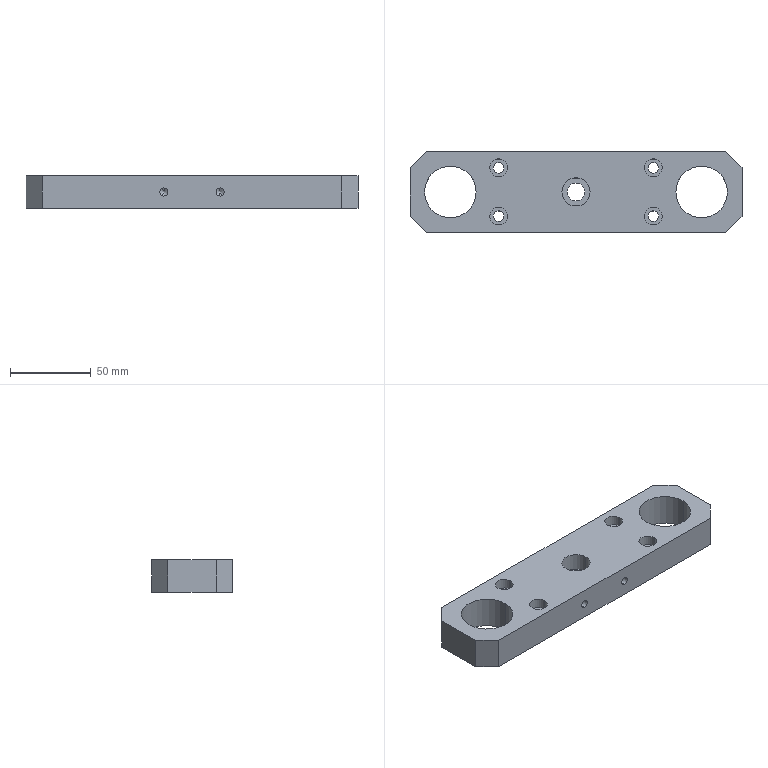Part | STEP file | BU-A04 | 1 solid | 47 faces | box 206 x 50 x 20 mm | volume 161458 mm3 | cylinder 28 | plane 15 | cone 4 | commonest cylinder face diameters 11 x10 6.5 x8 5 x4 32 x4 17.5 x2